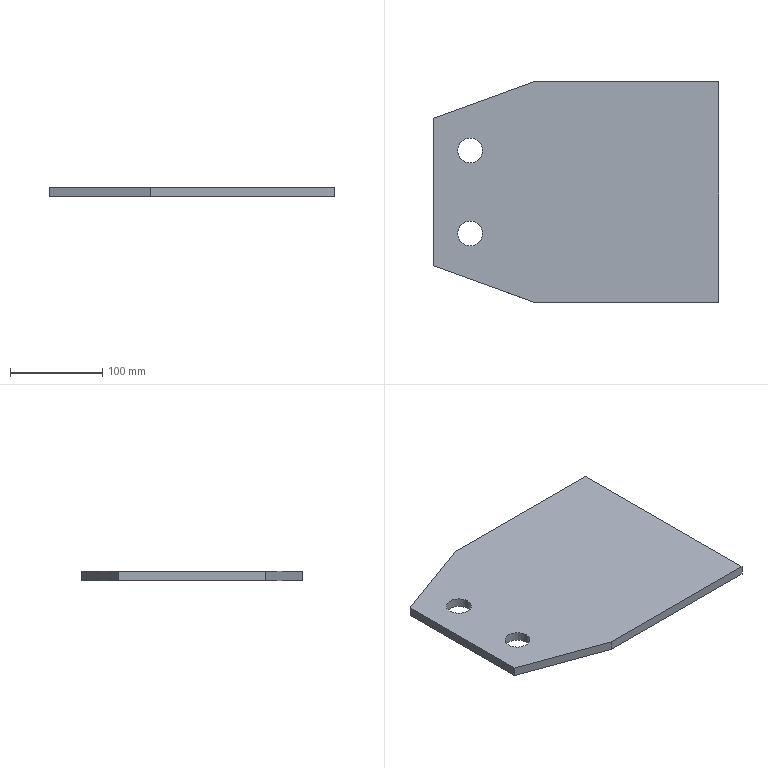Part | SolidWorks | features Extrusion 1, ICE 1 | 1 solid | 12 faces | box 310 x 240 x 10 mm | volume 688549 mm3 | plane 8 | cylinder 4 | commonest cylinder face diameters 27 x4
STEP:
#1=CARTESIAN_POINT('',(-128.5,45.,0.));
#2=VERTEX_POINT('',#1);
#3=CARTESIAN_POINT('',(-101.5,45.,0.));
#4=VERTEX_POINT('',#3);
#5=CARTESIAN_POINT('',(-115.,45.,0.));
#6=DIRECTION('',(0.,0.,1.));
#7=DIRECTION('',(1.,0.,0.));
#8=AXIS2_PLACEMENT_3D('',#5,#6,#7);
#9=CIRCLE('',#8,13.5);
#10=EDGE_CURVE('',#2,#4,#9,.T.);
#11=ORIENTED_EDGE('',*,*,#10,.F.);
#12=CARTESIAN_POINT('',(-128.5,45.,10.));
#13=VERTEX_POINT('',#12);
#14=CARTESIAN_POINT('',(-128.5,45.,0.));
#15=DIRECTION('',(0.,0.,1.));
#16=VECTOR('',#15,1000.);
#17=LINE('',#14,#16);
#18=EDGE_CURVE('',#2,#13,#17,.T.);
#19=ORIENTED_EDGE('',*,*,#18,.T.);
#20=CARTESIAN_POINT('',(-101.5,45.,10.));
#21=VERTEX_POINT('',#20);
#22=CARTESIAN_POINT('',(-115.,45.,10.));
#23=DIRECTION('',(0.,0.,1.));
#24=DIRECTION('',(1.,0.,0.));
#25=AXIS2_PLACEMENT_3D('',#22,#23,#24);
#26=CIRCLE('',#25,13.5);
#27=EDGE_CURVE('',#13,#21,#26,.T.);
#28=ORIENTED_EDGE('',*,*,#27,.T.);
#29=CARTESIAN_POINT('',(-101.5,45.,0.));
#30=DIRECTION('',(0.,0.,1.));
#31=VECTOR('',#30,1000.);
#32=LINE('',#29,#31);
#33=EDGE_CURVE('',#4,#21,#32,.T.);
#34=ORIENTED_EDGE('',*,*,#33,.F.);
#35=EDGE_LOOP('',(#11,#19,#28,#34));
#36=FACE_OUTER_BOUND('',#35,.T.);
#37=CARTESIAN_POINT('',(-115.,45.,0.));
#38=DIRECTION('',(0.,0.,1.));
#39=DIRECTION('',(1.,0.,0.));
#40=AXIS2_PLACEMENT_3D('',#37,#38,#39);
#41=CYLINDRICAL_SURFACE('',#40,13.5);
#42=ADVANCED_FACE('',(#36),#41,.F.);
#43=CARTESIAN_POINT('',(-128.5,-45.,0.));
#44=VERTEX_POINT('',#43);
#45=CARTESIAN_POINT('',(-101.5,-45.,0.));
#46=VERTEX_POINT('',#45);
#47=CARTESIAN_POINT('',(-115.,-45.,0.));
#48=DIRECTION('',(0.,0.,1.));
#49=DIRECTION('',(1.,0.,0.));
#50=AXIS2_PLACEMENT_3D('',#47,#48,#49);
#51=CIRCLE('',#50,13.5);
#52=EDGE_CURVE('',#44,#46,#51,.T.);
#53=ORIENTED_EDGE('',*,*,#52,.F.);
#54=CARTESIAN_POINT('',(-128.5,-45.,10.));
#55=VERTEX_POINT('',#54);
#56=CARTESIAN_POINT('',(-128.5,-45.,0.));
#57=DIRECTION('',(0.,0.,1.));
#58=VECTOR('',#57,1000.);
#59=LINE('',#56,#58);
#60=EDGE_CURVE('',#44,#55,#59,.T.);
#61=ORIENTED_EDGE('',*,*,#60,.T.);
#62=CARTESIAN_POINT('',(-101.5,-45.,10.));
#63=VERTEX_POINT('',#62);
#64=CARTESIAN_POINT('',(-115.,-45.,10.));
#65=DIRECTION('',(0.,0.,1.));
#66=DIRECTION('',(1.,0.,0.));
#67=AXIS2_PLACEMENT_3D('',#64,#65,#66);
#68=CIRCLE('',#67,13.5);
#69=EDGE_CURVE('',#55,#63,#68,.T.);
#70=ORIENTED_EDGE('',*,*,#69,.T.);
#71=CARTESIAN_POINT('',(-101.5,-45.,0.));
#72=DIRECTION('',(0.,0.,1.));
#73=VECTOR('',#72,1000.);
#74=LINE('',#71,#73);
#75=EDGE_CURVE('',#46,#63,#74,.T.);
#76=ORIENTED_EDGE('',*,*,#75,.F.);
#77=EDGE_LOOP('',(#53,#61,#70,#76));
#78=FACE_OUTER_BOUND('',#77,.T.);
#79=CARTESIAN_POINT('',(-115.,-45.,0.));
#80=DIRECTION('',(0.,0.,1.));
#81=DIRECTION('',(1.,0.,0.));
#82=AXIS2_PLACEMENT_3D('',#79,#80,#81);
#83=CYLINDRICAL_SURFACE('',#82,13.5);
#84=ADVANCED_FACE('',(#78),#83,.F.);
#85=CARTESIAN_POINT('',(-155.,80.,0.));
#86=VERTEX_POINT('',#85);
#87=CARTESIAN_POINT('',(-155.,-80.,0.));
#88=VERTEX_POINT('',#87);
#89=CARTESIAN_POINT('',(-155.,120.,0.));
#90=DIRECTION('',(0.,-1.,0.));
#91=VECTOR('',#90,1000.);
#92=LINE('',#89,#91);
#93=EDGE_CURVE('',#86,#88,#92,.T.);
#94=ORIENTED_EDGE('',*,*,#93,.T.);
#95=CARTESIAN_POINT('',(-155.,-80.,10.));
#96=VERTEX_POINT('',#95);
#97=CARTESIAN_POINT('',(-155.,-80.,0.));
#98=DIRECTION('',(0.,0.,1.));
#99=VECTOR('',#98,1000.);
#100=LINE('',#97,#99);
#101=EDGE_CURVE('',#88,#96,#100,.T.);
#102=ORIENTED_EDGE('',*,*,#101,.T.);
#103=CARTESIAN_POINT('',(-155.,80.,10.));
#104=VERTEX_POINT('',#103);
#105=CARTESIAN_POINT('',(-155.,120.,10.));
#106=DIRECTION('',(0.,-1.,0.));
#107=VECTOR('',#106,1000.);
#108=LINE('',#105,#107);
#109=EDGE_CURVE('',#104,#96,#108,.T.);
#110=ORIENTED_EDGE('',*,*,#109,.F.);
#111=CARTESIAN_POINT('',(-155.,80.,0.));
#112=DIRECTION('',(0.,0.,1.));
#113=VECTOR('',#112,1000.);
#114=LINE('',#111,#113);
#115=EDGE_CURVE('',#86,#104,#114,.T.);
#116=ORIENTED_EDGE('',*,*,#115,.F.);
#117=EDGE_LOOP('',(#94,#102,#110,#116));
#118=FACE_OUTER_BOUND('',#117,.T.);
#119=CARTESIAN_POINT('',(-155.,120.,10.));
#120=DIRECTION('',(1.,0.,0.));
#121=DIRECTION('',(0.,0.,-1.));
#122=AXIS2_PLACEMENT_3D('',#119,#120,#121);
#123=PLANE('',#122);
#124=ADVANCED_FACE('',(#118),#123,.F.);
#125=CARTESIAN_POINT('',(-45.,-120.,10.));
#126=VERTEX_POINT('',#125);
#127=CARTESIAN_POINT('',(155.,-120.,10.));
#128=VERTEX_POINT('',#127);
#129=CARTESIAN_POINT('',(155.,-120.,10.));
#130=DIRECTION('',(1.,0.,0.));
#131=VECTOR('',#130,1000.);
#132=LINE('',#129,#131);
#133=EDGE_CURVE('',#126,#128,#132,.T.);
#134=ORIENTED_EDGE('',*,*,#133,.F.);
#135=CARTESIAN_POINT('',(-45.,-120.,0.));
#136=VERTEX_POINT('',#135);
#137=CARTESIAN_POINT('',(-45.,-120.,0.));
#138=DIRECTION('',(0.,0.,1.));
#139=VECTOR('',#138,1000.);
#140=LINE('',#137,#139);
#141=EDGE_CURVE('',#136,#126,#140,.T.);
#142=ORIENTED_EDGE('',*,*,#141,.F.);
#143=CARTESIAN_POINT('',(155.,-120.,0.));
#144=VERTEX_POINT('',#143);
#145=CARTESIAN_POINT('',(155.,-120.,0.));
#146=DIRECTION('',(1.,0.,0.));
#147=VECTOR('',#146,1000.);
#148=LINE('',#145,#147);
#149=EDGE_CURVE('',#136,#144,#148,.T.);
#150=ORIENTED_EDGE('',*,*,#149,.T.);
#151=CARTESIAN_POINT('',(155.,-120.,10.));
#152=DIRECTION('',(0.,0.,-1.));
#153=VECTOR('',#152,1000.);
#154=LINE('',#151,#153);
#155=EDGE_CURVE('',#128,#144,#154,.T.);
#156=ORIENTED_EDGE('',*,*,#155,.F.);
#157=EDGE_LOOP('',(#134,#142,#150,#156));
#158=FACE_OUTER_BOUND('',#157,.T.);
#159=CARTESIAN_POINT('',(155.,-120.,10.));
#160=DIRECTION('',(0.,1.,0.));
#161=DIRECTION('',(-1.,0.,0.));
#162=AXIS2_PLACEMENT_3D('',#159,#160,#161);
#163=PLANE('',#162);
#164=ADVANCED_FACE('',(#158),#163,.F.);
#165=CARTESIAN_POINT('',(155.,120.,0.));
#166=VERTEX_POINT('',#165);
#167=CARTESIAN_POINT('',(155.,120.,0.));
#168=DIRECTION('',(0.,1.,0.));
#169=VECTOR('',#168,1000.);
#170=LINE('',#167,#169);
#171=EDGE_CURVE('',#144,#166,#170,.T.);
#172=ORIENTED_EDGE('',*,*,#171,.T.);
#173=CARTESIAN_POINT('',(155.,120.,10.));
#174=VERTEX_POINT('',#173);
#175=CARTESIAN_POINT('',(155.,120.,10.));
#176=DIRECTION('',(0.,0.,-1.));
#177=VECTOR('',#176,1000.);
#178=LINE('',#175,#177);
#179=EDGE_CURVE('',#174,#166,#178,.T.);
#180=ORIENTED_EDGE('',*,*,#179,.F.);
#181=CARTESIAN_POINT('',(155.,120.,10.));
#182=DIRECTION('',(0.,1.,0.));
#183=VECTOR('',#182,1000.);
#184=LINE('',#181,#183);
#185=EDGE_CURVE('',#128,#174,#184,.T.);
#186=ORIENTED_EDGE('',*,*,#185,.F.);
#187=ORIENTED_EDGE('',*,*,#155,.T.);
#188=EDGE_LOOP('',(#172,#180,#186,#187));
#189=FACE_OUTER_BOUND('',#188,.T.);
#190=CARTESIAN_POINT('',(155.,120.,10.));
#191=DIRECTION('',(-1.,0.,0.));
#192=DIRECTION('',(0.,-1.,0.));
#193=AXIS2_PLACEMENT_3D('',#190,#191,#192);
#194=PLANE('',#193);
#195=ADVANCED_FACE('',(#189),#194,.F.);
#196=CARTESIAN_POINT('',(-45.,120.,0.));
#197=VERTEX_POINT('',#196);
#198=CARTESIAN_POINT('',(155.,120.,0.));
#199=DIRECTION('',(-1.,0.,0.));
#200=VECTOR('',#199,1000.);
#201=LINE('',#198,#200);
#202=EDGE_CURVE('',#166,#197,#201,.T.);
#203=ORIENTED_EDGE('',*,*,#202,.T.);
#204=CARTESIAN_POINT('',(-45.,120.,10.));
#205=VERTEX_POINT('',#204);
#206=CARTESIAN_POINT('',(-45.,120.,0.));
#207=DIRECTION('',(0.,0.,1.));
#208=VECTOR('',#207,1000.);
#209=LINE('',#206,#208);
#210=EDGE_CURVE('',#197,#205,#209,.T.);
#211=ORIENTED_EDGE('',*,*,#210,.T.);
#212=CARTESIAN_POINT('',(155.,120.,10.));
#213=DIRECTION('',(-1.,0.,0.));
#214=VECTOR('',#213,1000.);
#215=LINE('',#212,#214);
#216=EDGE_CURVE('',#174,#205,#215,.T.);
#217=ORIENTED_EDGE('',*,*,#216,.F.);
#218=ORIENTED_EDGE('',*,*,#179,.T.);
#219=EDGE_LOOP('',(#203,#211,#217,#218));
#220=FACE_OUTER_BOUND('',#219,.T.);
#221=CARTESIAN_POINT('',(155.,120.,10.));
#222=DIRECTION('',(0.,-1.,0.));
#223=DIRECTION('',(1.,0.,0.));
#224=AXIS2_PLACEMENT_3D('',#221,#222,#223);
#225=PLANE('',#224);
#226=ADVANCED_FACE('',(#220),#225,.F.);
#227=CARTESIAN_POINT('',(-115.,45.,10.));
#228=DIRECTION('',(0.,0.,1.));
#229=DIRECTION('',(1.,0.,0.));
#230=AXIS2_PLACEMENT_3D('',#227,#228,#229);
#231=CIRCLE('',#230,13.5);
#232=EDGE_CURVE('',#21,#13,#231,.T.);
#233=ORIENTED_EDGE('',*,*,#232,.F.);
#234=ORIENTED_EDGE('',*,*,#27,.F.);
#235=EDGE_LOOP('',(#233,#234));
#236=FACE_BOUND('',#235,.T.);
#237=CARTESIAN_POINT('',(-115.,-45.,10.));
#238=DIRECTION('',(0.,0.,1.));
#239=DIRECTION('',(1.,0.,0.));
#240=AXIS2_PLACEMENT_3D('',#237,#238,#239);
#241=CIRCLE('',#240,13.5);
#242=EDGE_CURVE('',#63,#55,#241,.T.);
#243=ORIENTED_EDGE('',*,*,#242,.F.);
#244=ORIENTED_EDGE('',*,*,#69,.F.);
#245=EDGE_LOOP('',(#243,#244));
#246=FACE_BOUND('',#245,.T.);
#247=ORIENTED_EDGE('',*,*,#109,.T.);
#248=CARTESIAN_POINT('',(-155.,-80.,10.));
#249=DIRECTION('',(-0.9398,0.3417,0.));
#250=VECTOR('',#249,1000.);
#251=LINE('',#248,#250);
#252=EDGE_CURVE('',#126,#96,#251,.T.);
#253=ORIENTED_EDGE('',*,*,#252,.F.);
#254=ORIENTED_EDGE('',*,*,#133,.T.);
#255=ORIENTED_EDGE('',*,*,#185,.T.);
#256=ORIENTED_EDGE('',*,*,#216,.T.);
#257=CARTESIAN_POINT('',(-155.,80.,10.));
#258=DIRECTION('',(0.9398,0.3417,0.));
#259=VECTOR('',#258,1000.);
#260=LINE('',#257,#259);
#261=EDGE_CURVE('',#104,#205,#260,.T.);
#262=ORIENTED_EDGE('',*,*,#261,.F.);
#263=EDGE_LOOP('',(#247,#253,#254,#255,#256,#262));
#264=FACE_OUTER_BOUND('',#263,.T.);
#265=CARTESIAN_POINT('',(0.,0.,10.));
#266=DIRECTION('',(0.,0.,-1.));
#267=DIRECTION('',(-1.,0.,0.));
#268=AXIS2_PLACEMENT_3D('',#265,#266,#267);
#269=PLANE('',#268);
#270=ADVANCED_FACE('',(#236,#246,#264),#269,.F.);
#271=CARTESIAN_POINT('',(-155.,-80.,0.));
#272=DIRECTION('',(-0.9398,0.3417,0.));
#273=VECTOR('',#272,1000.);
#274=LINE('',#271,#273);
#275=EDGE_CURVE('',#136,#88,#274,.T.);
#276=ORIENTED_EDGE('',*,*,#275,.T.);
#277=ORIENTED_EDGE('',*,*,#93,.F.);
#278=CARTESIAN_POINT('',(-155.,80.,0.));
#279=DIRECTION('',(0.9398,0.3417,0.));
#280=VECTOR('',#279,1000.);
#281=LINE('',#278,#280);
#282=EDGE_CURVE('',#86,#197,#281,.T.);
#283=ORIENTED_EDGE('',*,*,#282,.T.);
#284=ORIENTED_EDGE('',*,*,#202,.F.);
#285=ORIENTED_EDGE('',*,*,#171,.F.);
#286=ORIENTED_EDGE('',*,*,#149,.F.);
#287=EDGE_LOOP('',(#276,#277,#283,#284,#285,#286));
#288=FACE_OUTER_BOUND('',#287,.T.);
#289=CARTESIAN_POINT('',(-115.,45.,0.));
#290=DIRECTION('',(0.,0.,1.));
#291=DIRECTION('',(1.,0.,0.));
#292=AXIS2_PLACEMENT_3D('',#289,#290,#291);
#293=CIRCLE('',#292,13.5);
#294=EDGE_CURVE('',#4,#2,#293,.T.);
#295=ORIENTED_EDGE('',*,*,#294,.T.);
#296=ORIENTED_EDGE('',*,*,#10,.T.);
#297=EDGE_LOOP('',(#295,#296));
#298=FACE_BOUND('',#297,.T.);
#299=CARTESIAN_POINT('',(-115.,-45.,0.));
#300=DIRECTION('',(0.,0.,1.));
#301=DIRECTION('',(1.,0.,0.));
#302=AXIS2_PLACEMENT_3D('',#299,#300,#301);
#303=CIRCLE('',#302,13.5);
#304=EDGE_CURVE('',#46,#44,#303,.T.);
#305=ORIENTED_EDGE('',*,*,#304,.T.);
#306=ORIENTED_EDGE('',*,*,#52,.T.);
#307=EDGE_LOOP('',(#305,#306));
#308=FACE_BOUND('',#307,.T.);
#309=CARTESIAN_POINT('',(0.,0.,0.));
#310=DIRECTION('',(0.,0.,-1.));
#311=DIRECTION('',(-1.,0.,0.));
#312=AXIS2_PLACEMENT_3D('',#309,#310,#311);
#313=PLANE('',#312);
#314=ADVANCED_FACE('',(#288,#298,#308),#313,.T.);
#315=ORIENTED_EDGE('',*,*,#60,.F.);
#316=ORIENTED_EDGE('',*,*,#304,.F.);
#317=ORIENTED_EDGE('',*,*,#75,.T.);
#318=ORIENTED_EDGE('',*,*,#242,.T.);
#319=EDGE_LOOP('',(#315,#316,#317,#318));
#320=FACE_OUTER_BOUND('',#319,.T.);
#321=CARTESIAN_POINT('',(-115.,-45.,0.));
#322=DIRECTION('',(0.,0.,1.));
#323=DIRECTION('',(1.,0.,0.));
#324=AXIS2_PLACEMENT_3D('',#321,#322,#323);
#325=CYLINDRICAL_SURFACE('',#324,13.5);
#326=ADVANCED_FACE('',(#320),#325,.F.);
#327=ORIENTED_EDGE('',*,*,#18,.F.);
#328=ORIENTED_EDGE('',*,*,#294,.F.);
#329=ORIENTED_EDGE('',*,*,#33,.T.);
#330=ORIENTED_EDGE('',*,*,#232,.T.);
#331=EDGE_LOOP('',(#327,#328,#329,#330));
#332=FACE_OUTER_BOUND('',#331,.T.);
#333=CARTESIAN_POINT('',(-115.,45.,0.));
#334=DIRECTION('',(0.,0.,1.));
#335=DIRECTION('',(1.,0.,0.));
#336=AXIS2_PLACEMENT_3D('',#333,#334,#335);
#337=CYLINDRICAL_SURFACE('',#336,13.5);
#338=ADVANCED_FACE('',(#332),#337,.F.);
#339=ORIENTED_EDGE('',*,*,#261,.T.);
#340=ORIENTED_EDGE('',*,*,#210,.F.);
#341=ORIENTED_EDGE('',*,*,#282,.F.);
#342=ORIENTED_EDGE('',*,*,#115,.T.);
#343=EDGE_LOOP('',(#339,#340,#341,#342));
#344=FACE_OUTER_BOUND('',#343,.T.);
#345=CARTESIAN_POINT('',(-155.,80.,0.));
#346=DIRECTION('',(0.3417,-0.9398,0.));
#347=DIRECTION('',(0.9398,0.3417,0.));
#348=AXIS2_PLACEMENT_3D('',#345,#346,#347);
#349=PLANE('',#348);
#350=ADVANCED_FACE('',(#344),#349,.F.);
#351=ORIENTED_EDGE('',*,*,#252,.T.);
#352=ORIENTED_EDGE('',*,*,#101,.F.);
#353=ORIENTED_EDGE('',*,*,#275,.F.);
#354=ORIENTED_EDGE('',*,*,#141,.T.);
#355=EDGE_LOOP('',(#351,#352,#353,#354));
#356=FACE_OUTER_BOUND('',#355,.T.);
#357=CARTESIAN_POINT('',(-155.,-80.,0.));
#358=DIRECTION('',(0.3417,0.9398,0.));
#359=DIRECTION('',(-0.9398,0.3417,0.));
#360=AXIS2_PLACEMENT_3D('',#357,#358,#359);
#361=PLANE('',#360);
#362=ADVANCED_FACE('',(#356),#361,.F.);
#363=CLOSED_SHELL('',(#42,#84,#124,#164,#195,#226,#270,#314,#326,#338,#350,#362));
#364=MANIFOLD_SOLID_BREP('',#363);
#365=CARTESIAN_POINT('',(0.,0.,0.));
#366=DIRECTION('',(0.,0.,1.));
#367=DIRECTION('',(1.,0.,0.));
#368=AXIS2_PLACEMENT_3D('',#365,#366,#367);
#369=(LENGTH_UNIT()NAMED_UNIT(*)SI_UNIT(.MILLI.,.METRE.));
#370=UNCERTAINTY_MEASURE_WITH_UNIT(LENGTH_MEASURE(0.00001),#369,'','');
#371=(NAMED_UNIT(*)PLANE_ANGLE_UNIT()SI_UNIT($,.RADIAN.));
#372=(NAMED_UNIT(*)SI_UNIT($,.STERADIAN.)SOLID_ANGLE_UNIT());
#373=(GEOMETRIC_REPRESENTATION_CONTEXT(3)GLOBAL_UNCERTAINTY_ASSIGNED_CONTEXT((#370))GLOBAL_UNIT_ASSIGNED_CONTEXT((#369,#371,#372))REPRESENTATION_CONTEXT('',''));
#374=ADVANCED_BREP_SHAPE_REPRESENTATION('',(#364,#368),#373);